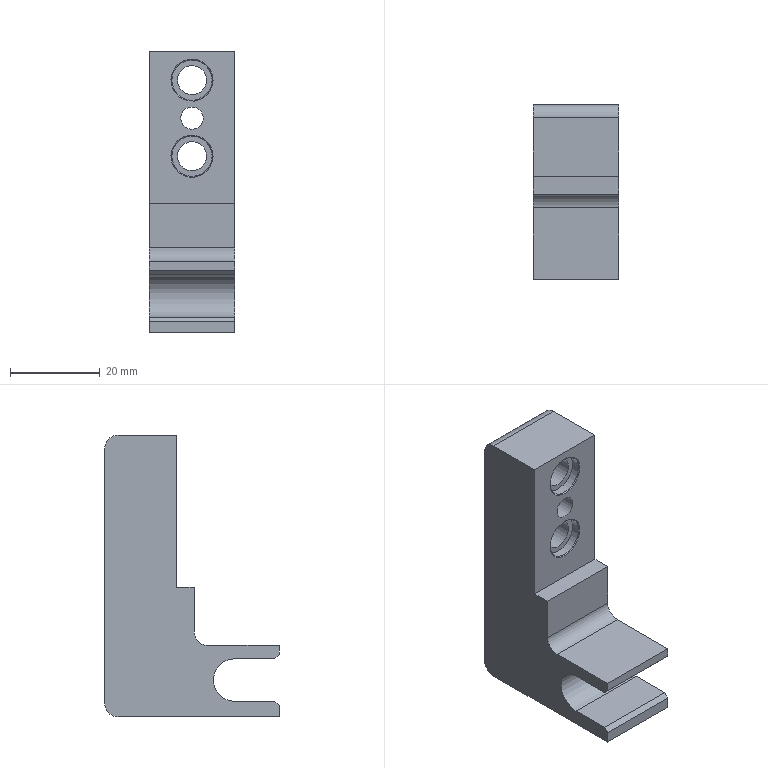Part | STEP file | SN10_012_001_GARRA | 1 solid | 28 faces | box 19 x 39 x 63 mm | volume 23093 mm3 | plane 17 | cylinder 9 | cone 2 | commonest cylinder face diameters 6 x3 6.5 x2 9 x2 5 x1 9.5 x1